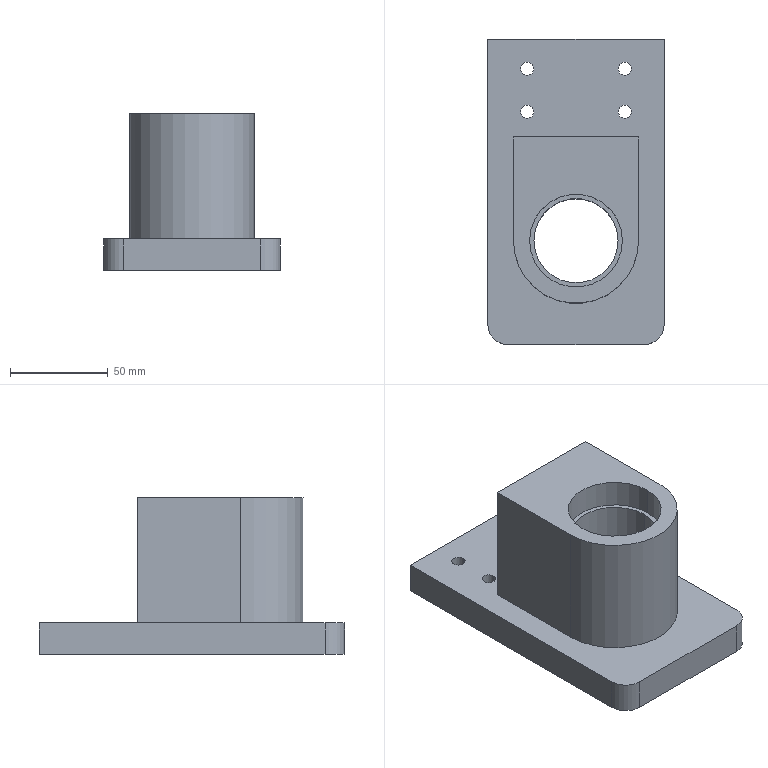NC program | NX | posted with a generic post | part box 90 x 156 x 80 mm
Lines 1963 to 2108 of 2108:
(FLOOR_WALL , TOOL : D50面刀)
N3918 T03 M6
N3920 G54
N3922 G17 G0 G90 X115.65 Y-44.425 S2000 M3
N3924 G43 Z30. H3
N3926 Z3.
N3928 G94 G1 Z0. F600.
N3930 G3 X103. Y-32.077 R12.5
N3932 G1 X-103. Y-34.564
N3934 Y-4.934
N3936 X103. Y-2.447
N3938 Y27.183
N3940 X-103. Y24.696
N3942 G3 X-115.348 Y12.046 R12.5
N3944 G1 Z3.
N3946 G0 Z30.
N3948 M5
(PLANAR_MILL_5_COPY , TOOL : D10-30-D10-75-3T-FINISH)
N3950 T06 M6
N3952 G54
N3954 G17 G0 G90 X23. Y-16.63 S3000 M3
N3956 G43 Z30. H6
N3958 Z-12.
N3960 G94 G1 Z-14. F1000.
N3962 Y-16.75
N3964 G3 X25. Y-18.75 R2.
N3966 X43.75 Y0. R18.75
N3968 X25. Y-18.75 R-18.75
N3970 X27. Y-16.75 R2.
N3972 G1 X23.
N3974 G3 X25. Y-18.75 R2.
N3976 X43.75 Y0. R18.75
N3978 X25. Y-18.75 R-18.75
N3980 X27. Y-16.75 R2.
N3982 G1 Y-16.63
N3984 Z-12.
N3986 G0 Z30.
N3988 M5
(PLANAR_MILL_6 , TOOL : 倒角D10-90度)
N3990 T04 M6
N3992 G54
N3994 G17 G0 G90 X-3. Y-49. S3000 M3
N3996 G43 Z30. H4
N3998 Z0.
N4000 G94 G1 Z-2. F1000.
N4002 G3 X-5. Y-47. R2.
N4004 G1 X-78.
N4006 G2 X-80. Y-45. R2.
N4008 G1 Y45.
N4010 G2 X-78. Y47. R2.
N4012 G1 X68.
N4014 G2 X80. Y35. R12.
N4016 G1 Y-35.
N4018 G2 X68. Y-47. R12.
N4020 G1 X-5.
N4022 G3 X-7. Y-49. R2.
N4024 G1 Z0.
N4026 G0 Z30.
(PLANAR_MILL_6_COPY , TOOL : 倒角D10-90度)
N4028 X23. Y-19.648
N4030 Z0.
N4032 G1 Z-2.
N4034 Y-19.75
N4036 G3 X25. Y-21.75 R2.
N4038 X46.75 Y0. R21.75
N4040 X25. Y-21.75 R-21.75
N4042 X27. Y-19.75 R2.
N4044 G1 Y-19.648
N4046 Z0.
N4048 G0 Z30.
(PLANAR_MILL_6_COPY_1 , TOOL : 倒角D10-90度)
N4050 Y15.37
N4052 Z-16.
N4054 G1 Z-18.
N4056 Y15.5
N4058 G3 X25. Y17.5 R2.
N4060 X7.5 Y0. R17.5
N4062 X25. Y17.5 R-17.5
N4064 X23. Y15.5 R2.
N4066 G1 Y15.37
N4068 Z-16.
N4070 G0 Z30.
(DRILLING , TOOL : 倒角D10-90度)
N4072 X-63. Y25. S1200
N4074 G81 G98 Z-1.5 F100. R3.
N4076 X-41.
N4078 Y-25.
N4080 X-63.
N4082 G80
N4084 G0 X-63. Y-25. Z30.
N4086 M5
(DRILLING_COPY , TOOL : 钻头D6.8-73-105)
N4088 T07 M6
N4090 G54
N4092 G17 G0 G90 X-63. Y25. S1200 M3
N4094 G43 Z30. H7
N4096 G94 G83 G98 Z-20. F100. Q2. R3.
N4098 X-41.
N4100 Y-25.
N4102 X-63.
N4104 G80
N4106 G0 X-63. Y-25. Z30.
N4108 M5
(DRILLING_COPY_1 , TOOL : 倒角D10-90度)
N4110 T04 M6
N4112 G54
N4114 G17 G0 G90 X-63. Y25. S1200 M3
N4116 G43 Z30. H4
N4118 G94 G81 G98 Z-4. F100. R3.
N4120 X-41.
N4122 Y-25.
N4124 X-63.
N4126 G80
N4128 G0 X-63. Y-25. Z30.
N4130 M5
(DRILLING_COPY_COPY , TOOL : 上排M8-28-D6.2-70)
N4132 T07 M6
N4134 G54
N4136 G17 G0 G90 X-63. Y25. S300 M3
N4138 G43 Z30. H7
N4140 G84 G94 G98 Z-10. F375. R3.
N4142 X-41.
N4144 Y-25.
N4146 X-63.
N4148 G80
N4150 G0 X-63. Y-25. Z30.
N4152 M5
N4154 M2